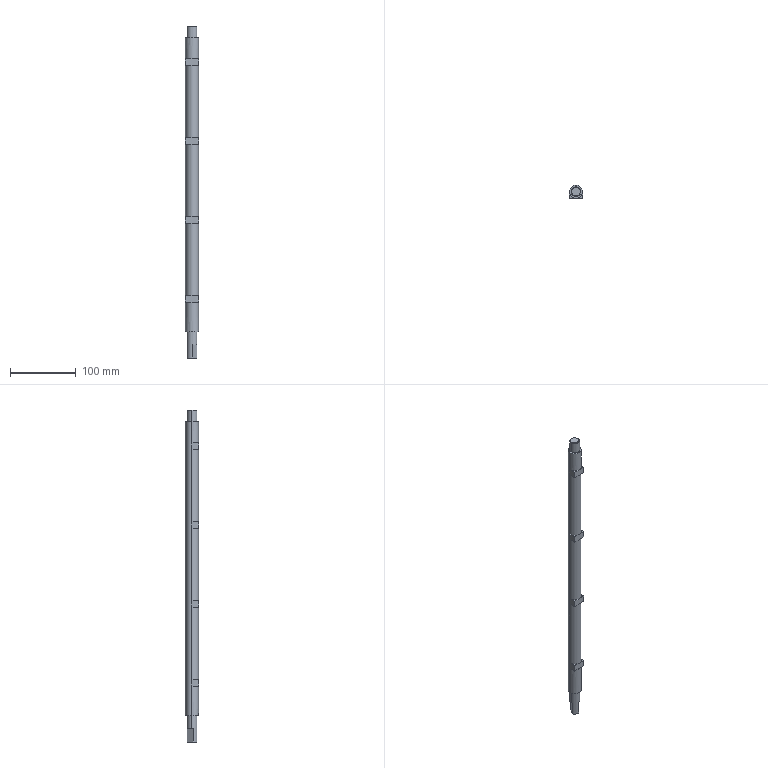Part | SolidWorks | features BaseBody 1 | 1 solid | 48 faces | box 20 x 20 x 505 mm | volume 151599 mm3 | plane 36 | cylinder 10 | cone 2 | commonest cylinder face diameters 20 x6 15 x4
STEP:
#1=CARTESIAN_POINT('',(-1.019,7.43,-20.));
#2=VERTEX_POINT('',#1);
#3=CARTESIAN_POINT('',(-7.5,0.,-20.));
#4=VERTEX_POINT('',#3);
#5=CARTESIAN_POINT('',(0.,0.,-20.));
#6=DIRECTION('',(0.,0.,1.));
#7=DIRECTION('',(1.,0.,0.));
#8=AXIS2_PLACEMENT_3D('',#5,#6,#7);
#9=CIRCLE('',#8,7.5);
#10=EDGE_CURVE('',#2,#4,#9,.T.);
#11=ORIENTED_EDGE('',*,*,#10,.T.);
#12=CARTESIAN_POINT('',(-7.5,0.,0.));
#13=VERTEX_POINT('',#12);
#14=CARTESIAN_POINT('',(-7.5,0.,0.));
#15=DIRECTION('',(0.,0.,1.));
#16=VECTOR('',#15,1000.);
#17=LINE('',#14,#16);
#18=EDGE_CURVE('',#4,#13,#17,.T.);
#19=ORIENTED_EDGE('',*,*,#18,.T.);
#20=CARTESIAN_POINT('',(7.5,0.,0.));
#21=VERTEX_POINT('',#20);
#22=CARTESIAN_POINT('',(0.,0.,0.));
#23=DIRECTION('',(0.,0.,1.));
#24=DIRECTION('',(1.,0.,0.));
#25=AXIS2_PLACEMENT_3D('',#22,#23,#24);
#26=CIRCLE('',#25,7.5);
#27=EDGE_CURVE('',#21,#13,#26,.T.);
#28=ORIENTED_EDGE('',*,*,#27,.F.);
#29=CARTESIAN_POINT('',(7.5,0.,-20.));
#30=VERTEX_POINT('',#29);
#31=CARTESIAN_POINT('',(7.5,0.,0.));
#32=DIRECTION('',(0.,0.,1.));
#33=VECTOR('',#32,1000.);
#34=LINE('',#31,#33);
#35=EDGE_CURVE('',#30,#21,#34,.T.);
#36=ORIENTED_EDGE('',*,*,#35,.F.);
#37=CARTESIAN_POINT('',(7.271,1.838,-20.));
#38=VERTEX_POINT('',#37);
#39=CARTESIAN_POINT('',(0.,0.,-20.));
#40=DIRECTION('',(0.,0.,1.));
#41=DIRECTION('',(1.,0.,0.));
#42=AXIS2_PLACEMENT_3D('',#39,#40,#41);
#43=CIRCLE('',#42,7.5);
#44=EDGE_CURVE('',#30,#38,#43,.T.);
#45=ORIENTED_EDGE('',*,*,#44,.T.);
#46=CARTESIAN_POINT('',(7.271,1.838,-40.));
#47=VERTEX_POINT('',#46);
#48=CARTESIAN_POINT('',(7.271,1.838,0.));
#49=DIRECTION('',(0.,0.,-1.));
#50=VECTOR('',#49,1000.);
#51=LINE('',#48,#50);
#52=EDGE_CURVE('',#38,#47,#51,.T.);
#53=ORIENTED_EDGE('',*,*,#52,.T.);
#54=CARTESIAN_POINT('',(-1.019,7.43,-40.));
#55=VERTEX_POINT('',#54);
#56=CARTESIAN_POINT('',(0.,0.,-40.));
#57=DIRECTION('',(0.,0.,-1.));
#58=DIRECTION('',(1.,0.,0.));
#59=AXIS2_PLACEMENT_3D('',#56,#57,#58);
#60=CIRCLE('',#59,7.5);
#61=EDGE_CURVE('',#55,#47,#60,.T.);
#62=ORIENTED_EDGE('',*,*,#61,.F.);
#63=CARTESIAN_POINT('',(-1.019,7.43,0.));
#64=DIRECTION('',(0.,0.,1.));
#65=VECTOR('',#64,1000.);
#66=LINE('',#63,#65);
#67=EDGE_CURVE('',#55,#2,#66,.T.);
#68=ORIENTED_EDGE('',*,*,#67,.T.);
#69=EDGE_LOOP('',(#11,#19,#28,#36,#45,#53,#62,#68));
#70=FACE_OUTER_BOUND('',#69,.T.);
#71=CARTESIAN_POINT('',(0.,0.,0.));
#72=DIRECTION('',(0.,0.,1.));
#73=DIRECTION('',(1.,0.,0.));
#74=AXIS2_PLACEMENT_3D('',#71,#72,#73);
#75=CYLINDRICAL_SURFACE('',#74,7.5);
#76=ADVANCED_FACE('',(#70),#75,.T.);
#77=CARTESIAN_POINT('',(-6.5,0.,465.));
#78=VERTEX_POINT('',#77);
#79=CARTESIAN_POINT('',(6.5,0.,465.));
#80=VERTEX_POINT('',#79);
#81=CARTESIAN_POINT('',(0.,0.,465.));
#82=DIRECTION('',(0.,0.,-1.));
#83=DIRECTION('',(-1.,0.,0.));
#84=AXIS2_PLACEMENT_3D('',#81,#82,#83);
#85=CIRCLE('',#84,6.5);
#86=EDGE_CURVE('',#78,#80,#85,.T.);
#87=ORIENTED_EDGE('',*,*,#86,.T.);
#88=CARTESIAN_POINT('',(7.5,0.,464.));
#89=VERTEX_POINT('',#88);
#90=CARTESIAN_POINT('',(7.,0.,464.5));
#91=DIRECTION('',(0.7071,0.,-0.7071));
#92=VECTOR('',#91,1000.);
#93=LINE('',#90,#92);
#94=EDGE_CURVE('',#80,#89,#93,.T.);
#95=ORIENTED_EDGE('',*,*,#94,.T.);
#96=CARTESIAN_POINT('',(-7.5,0.,464.));
#97=VERTEX_POINT('',#96);
#98=CARTESIAN_POINT('',(0.,0.,464.));
#99=DIRECTION('',(0.,0.,1.));
#100=DIRECTION('',(-1.,0.,0.));
#101=AXIS2_PLACEMENT_3D('',#98,#99,#100);
#102=CIRCLE('',#101,7.5);
#103=EDGE_CURVE('',#89,#97,#102,.T.);
#104=ORIENTED_EDGE('',*,*,#103,.T.);
#105=CARTESIAN_POINT('',(-7.,0.,464.5));
#106=DIRECTION('',(-0.7071,0.,-0.7071));
#107=VECTOR('',#106,1000.);
#108=LINE('',#105,#107);
#109=EDGE_CURVE('',#78,#97,#108,.T.);
#110=ORIENTED_EDGE('',*,*,#109,.F.);
#111=EDGE_LOOP('',(#87,#95,#104,#110));
#112=FACE_OUTER_BOUND('',#111,.T.);
#113=CARTESIAN_POINT('',(0.,0.,464.5));
#114=DIRECTION('',(0.,0.,-1.));
#115=DIRECTION('',(-1.,0.,0.));
#116=AXIS2_PLACEMENT_3D('',#113,#114,#115);
#117=CONICAL_SURFACE('',#116,7.,0.7854);
#118=ADVANCED_FACE('',(#112),#117,.T.);
#119=ORIENTED_EDGE('',*,*,#103,.F.);
#120=CARTESIAN_POINT('',(7.5,0.,447.));
#121=VERTEX_POINT('',#120);
#122=CARTESIAN_POINT('',(7.5,0.,447.));
#123=DIRECTION('',(0.,0.,-1.));
#124=VECTOR('',#123,1000.);
#125=LINE('',#122,#124);
#126=EDGE_CURVE('',#89,#121,#125,.T.);
#127=ORIENTED_EDGE('',*,*,#126,.T.);
#128=CARTESIAN_POINT('',(-7.5,0.,447.));
#129=VERTEX_POINT('',#128);
#130=CARTESIAN_POINT('',(0.,0.,447.));
#131=DIRECTION('',(0.,0.,-1.));
#132=DIRECTION('',(-1.,0.,0.));
#133=AXIS2_PLACEMENT_3D('',#130,#131,#132);
#134=CIRCLE('',#133,7.5);
#135=EDGE_CURVE('',#129,#121,#134,.T.);
#136=ORIENTED_EDGE('',*,*,#135,.F.);
#137=CARTESIAN_POINT('',(-7.5,0.,447.));
#138=DIRECTION('',(0.,0.,-1.));
#139=VECTOR('',#138,1000.);
#140=LINE('',#137,#139);
#141=EDGE_CURVE('',#97,#129,#140,.T.);
#142=ORIENTED_EDGE('',*,*,#141,.F.);
#143=EDGE_LOOP('',(#119,#127,#136,#142));
#144=FACE_OUTER_BOUND('',#143,.T.);
#145=CARTESIAN_POINT('',(0.,0.,447.));
#146=DIRECTION('',(0.,0.,-1.));
#147=DIRECTION('',(-1.,0.,0.));
#148=AXIS2_PLACEMENT_3D('',#145,#146,#147);
#149=CYLINDRICAL_SURFACE('',#148,7.5);
#150=ADVANCED_FACE('',(#144),#149,.T.);
#151=CARTESIAN_POINT('',(10.,0.,447.));
#152=VERTEX_POINT('',#151);
#153=CARTESIAN_POINT('',(-10.,0.,447.));
#154=VERTEX_POINT('',#153);
#155=CARTESIAN_POINT('',(0.,0.,447.));
#156=DIRECTION('',(0.,0.,1.));
#157=DIRECTION('',(-1.,0.,0.));
#158=AXIS2_PLACEMENT_3D('',#155,#156,#157);
#159=CIRCLE('',#158,10.);
#160=EDGE_CURVE('',#152,#154,#159,.T.);
#161=ORIENTED_EDGE('',*,*,#160,.F.);
#162=CARTESIAN_POINT('',(10.,0.,415.));
#163=VERTEX_POINT('',#162);
#164=CARTESIAN_POINT('',(10.,0.,0.));
#165=DIRECTION('',(0.,0.,-1.));
#166=VECTOR('',#165,1000.);
#167=LINE('',#164,#166);
#168=EDGE_CURVE('',#152,#163,#167,.T.);
#169=ORIENTED_EDGE('',*,*,#168,.T.);
#170=CARTESIAN_POINT('',(10.,0.,405.));
#171=VERTEX_POINT('',#170);
#172=CARTESIAN_POINT('',(10.,0.,0.));
#173=DIRECTION('',(0.,0.,1.));
#174=VECTOR('',#173,1000.);
#175=LINE('',#172,#174);
#176=EDGE_CURVE('',#171,#163,#175,.T.);
#177=ORIENTED_EDGE('',*,*,#176,.F.);
#178=CARTESIAN_POINT('',(10.,0.,295.));
#179=VERTEX_POINT('',#178);
#180=CARTESIAN_POINT('',(10.,0.,0.));
#181=DIRECTION('',(0.,0.,-1.));
#182=VECTOR('',#181,1000.);
#183=LINE('',#180,#182);
#184=EDGE_CURVE('',#171,#179,#183,.T.);
#185=ORIENTED_EDGE('',*,*,#184,.T.);
#186=CARTESIAN_POINT('',(10.,0.,285.));
#187=VERTEX_POINT('',#186);
#188=CARTESIAN_POINT('',(10.,0.,0.));
#189=DIRECTION('',(0.,0.,1.));
#190=VECTOR('',#189,1000.);
#191=LINE('',#188,#190);
#192=EDGE_CURVE('',#187,#179,#191,.T.);
#193=ORIENTED_EDGE('',*,*,#192,.F.);
#194=CARTESIAN_POINT('',(10.,0.,175.));
#195=VERTEX_POINT('',#194);
#196=CARTESIAN_POINT('',(10.,0.,0.));
#197=DIRECTION('',(0.,0.,-1.));
#198=VECTOR('',#197,1000.);
#199=LINE('',#196,#198);
#200=EDGE_CURVE('',#187,#195,#199,.T.);
#201=ORIENTED_EDGE('',*,*,#200,.T.);
#202=CARTESIAN_POINT('',(10.,0.,165.));
#203=VERTEX_POINT('',#202);
#204=CARTESIAN_POINT('',(10.,0.,0.));
#205=DIRECTION('',(0.,0.,1.));
#206=VECTOR('',#205,1000.);
#207=LINE('',#204,#206);
#208=EDGE_CURVE('',#203,#195,#207,.T.);
#209=ORIENTED_EDGE('',*,*,#208,.F.);
#210=CARTESIAN_POINT('',(10.,0.,55.));
#211=VERTEX_POINT('',#210);
#212=CARTESIAN_POINT('',(10.,0.,0.));
#213=DIRECTION('',(0.,0.,-1.));
#214=VECTOR('',#213,1000.);
#215=LINE('',#212,#214);
#216=EDGE_CURVE('',#203,#211,#215,.T.);
#217=ORIENTED_EDGE('',*,*,#216,.T.);
#218=CARTESIAN_POINT('',(10.,0.,45.));
#219=VERTEX_POINT('',#218);
#220=CARTESIAN_POINT('',(10.,0.,0.));
#221=DIRECTION('',(0.,0.,1.));
#222=VECTOR('',#221,1000.);
#223=LINE('',#220,#222);
#224=EDGE_CURVE('',#219,#211,#223,.T.);
#225=ORIENTED_EDGE('',*,*,#224,.F.);
#226=CARTESIAN_POINT('',(10.,0.,0.));
#227=VERTEX_POINT('',#226);
#228=CARTESIAN_POINT('',(10.,0.,0.));
#229=DIRECTION('',(0.,0.,-1.));
#230=VECTOR('',#229,1000.);
#231=LINE('',#228,#230);
#232=EDGE_CURVE('',#219,#227,#231,.T.);
#233=ORIENTED_EDGE('',*,*,#232,.T.);
#234=CARTESIAN_POINT('',(-10.,0.,0.));
#235=VERTEX_POINT('',#234);
#236=CARTESIAN_POINT('',(0.,0.,0.));
#237=DIRECTION('',(0.,0.,-1.));
#238=DIRECTION('',(-1.,0.,0.));
#239=AXIS2_PLACEMENT_3D('',#236,#237,#238);
#240=CIRCLE('',#239,10.);
#241=EDGE_CURVE('',#235,#227,#240,.T.);
#242=ORIENTED_EDGE('',*,*,#241,.F.);
#243=CARTESIAN_POINT('',(-10.,0.,45.));
#244=VERTEX_POINT('',#243);
#245=CARTESIAN_POINT('',(-10.,0.,0.));
#246=DIRECTION('',(0.,0.,-1.));
#247=VECTOR('',#246,1000.);
#248=LINE('',#245,#247);
#249=EDGE_CURVE('',#244,#235,#248,.T.);
#250=ORIENTED_EDGE('',*,*,#249,.F.);
#251=CARTESIAN_POINT('',(-10.,0.,55.));
#252=VERTEX_POINT('',#251);
#253=CARTESIAN_POINT('',(-10.,0.,0.));
#254=DIRECTION('',(0.,0.,1.));
#255=VECTOR('',#254,1000.);
#256=LINE('',#253,#255);
#257=EDGE_CURVE('',#244,#252,#256,.T.);
#258=ORIENTED_EDGE('',*,*,#257,.T.);
#259=CARTESIAN_POINT('',(-10.,0.,165.));
#260=VERTEX_POINT('',#259);
#261=CARTESIAN_POINT('',(-10.,0.,0.));
#262=DIRECTION('',(0.,0.,-1.));
#263=VECTOR('',#262,1000.);
#264=LINE('',#261,#263);
#265=EDGE_CURVE('',#260,#252,#264,.T.);
#266=ORIENTED_EDGE('',*,*,#265,.F.);
#267=CARTESIAN_POINT('',(-10.,0.,175.));
#268=VERTEX_POINT('',#267);
#269=CARTESIAN_POINT('',(-10.,0.,0.));
#270=DIRECTION('',(0.,0.,1.));
#271=VECTOR('',#270,1000.);
#272=LINE('',#269,#271);
#273=EDGE_CURVE('',#260,#268,#272,.T.);
#274=ORIENTED_EDGE('',*,*,#273,.T.);
#275=CARTESIAN_POINT('',(-10.,0.,285.));
#276=VERTEX_POINT('',#275);
#277=CARTESIAN_POINT('',(-10.,0.,0.));
#278=DIRECTION('',(0.,0.,-1.));
#279=VECTOR('',#278,1000.);
#280=LINE('',#277,#279);
#281=EDGE_CURVE('',#276,#268,#280,.T.);
#282=ORIENTED_EDGE('',*,*,#281,.F.);
#283=CARTESIAN_POINT('',(-10.,0.,295.));
#284=VERTEX_POINT('',#283);
#285=CARTESIAN_POINT('',(-10.,0.,0.));
#286=DIRECTION('',(0.,0.,1.));
#287=VECTOR('',#286,1000.);
#288=LINE('',#285,#287);
#289=EDGE_CURVE('',#276,#284,#288,.T.);
#290=ORIENTED_EDGE('',*,*,#289,.T.);
#291=CARTESIAN_POINT('',(-10.,0.,405.));
#292=VERTEX_POINT('',#291);
#293=CARTESIAN_POINT('',(-10.,0.,0.));
#294=DIRECTION('',(0.,0.,-1.));
#295=VECTOR('',#294,1000.);
#296=LINE('',#293,#295);
#297=EDGE_CURVE('',#292,#284,#296,.T.);
#298=ORIENTED_EDGE('',*,*,#297,.F.);
#299=CARTESIAN_POINT('',(-10.,0.,415.));
#300=VERTEX_POINT('',#299);
#301=CARTESIAN_POINT('',(-10.,0.,0.));
#302=DIRECTION('',(0.,0.,1.));
#303=VECTOR('',#302,1000.);
#304=LINE('',#301,#303);
#305=EDGE_CURVE('',#292,#300,#304,.T.);
#306=ORIENTED_EDGE('',*,*,#305,.T.);
#307=CARTESIAN_POINT('',(-10.,0.,0.));
#308=DIRECTION('',(0.,0.,-1.));
#309=VECTOR('',#308,1000.);
#310=LINE('',#307,#309);
#311=EDGE_CURVE('',#154,#300,#310,.T.);
#312=ORIENTED_EDGE('',*,*,#311,.F.);
#313=EDGE_LOOP('',(#161,#169,#177,#185,#193,#201,#209,#217,#225,#233,#242,#250,#258,#266,#274,#282,#290,#298,#306,#312));
#314=FACE_OUTER_BOUND('',#313,.T.);
#315=CARTESIAN_POINT('',(0.,0.,0.));
#316=DIRECTION('',(0.,0.,-1.));
#317=DIRECTION('',(-1.,0.,0.));
#318=AXIS2_PLACEMENT_3D('',#315,#316,#317);
#319=CYLINDRICAL_SURFACE('',#318,10.);
#320=ADVANCED_FACE('',(#314),#319,.T.);
#321=ORIENTED_EDGE('',*,*,#168,.F.);
#322=CARTESIAN_POINT('',(0.,0.,447.));
#323=DIRECTION('',(0.,0.,1.));
#324=DIRECTION('',(-1.,0.,0.));
#325=AXIS2_PLACEMENT_3D('',#322,#323,#324);
#326=CIRCLE('',#325,10.);
#327=EDGE_CURVE('',#154,#152,#326,.T.);
#328=ORIENTED_EDGE('',*,*,#327,.F.);
#329=ORIENTED_EDGE('',*,*,#311,.T.);
#330=CARTESIAN_POINT('',(0.,-10.,415.));
#331=VERTEX_POINT('',#330);
#332=CARTESIAN_POINT('',(0.,0.,415.));
#333=DIRECTION('',(0.,0.,1.));
#334=DIRECTION('',(-1.,0.,0.));
#335=AXIS2_PLACEMENT_3D('',#332,#333,#334);
#336=CIRCLE('',#335,10.);
#337=EDGE_CURVE('',#300,#331,#336,.T.);
#338=ORIENTED_EDGE('',*,*,#337,.T.);
#339=CARTESIAN_POINT('',(0.,0.,415.));
#340=DIRECTION('',(0.,0.,1.));
#341=DIRECTION('',(-1.,0.,0.));
#342=AXIS2_PLACEMENT_3D('',#339,#340,#341);
#343=CIRCLE('',#342,10.);
#344=EDGE_CURVE('',#331,#163,#343,.T.);
#345=ORIENTED_EDGE('',*,*,#344,.T.);
#346=EDGE_LOOP('',(#321,#328,#329,#338,#345));
#347=FACE_OUTER_BOUND('',#346,.T.);
#348=CARTESIAN_POINT('',(0.,0.,0.));
#349=DIRECTION('',(0.,0.,-1.));
#350=DIRECTION('',(-1.,0.,0.));
#351=AXIS2_PLACEMENT_3D('',#348,#349,#350);
#352=CYLINDRICAL_SURFACE('',#351,10.);
#353=ADVANCED_FACE('',(#347),#352,.T.);
#354=ORIENTED_EDGE('',*,*,#184,.F.);
#355=CARTESIAN_POINT('',(0.,-10.,405.));
#356=VERTEX_POINT('',#355);
#357=CARTESIAN_POINT('',(0.,0.,405.));
#358=DIRECTION('',(0.,0.,-1.));
#359=DIRECTION('',(-1.,0.,0.));
#360=AXIS2_PLACEMENT_3D('',#357,#358,#359);
#361=CIRCLE('',#360,10.);
#362=EDGE_CURVE('',#171,#356,#361,.T.);
#363=ORIENTED_EDGE('',*,*,#362,.T.);
#364=CARTESIAN_POINT('',(0.,0.,405.));
#365=DIRECTION('',(0.,0.,-1.));
#366=DIRECTION('',(-1.,0.,0.));
#367=AXIS2_PLACEMENT_3D('',#364,#365,#366);
#368=CIRCLE('',#367,10.);
#369=EDGE_CURVE('',#356,#292,#368,.T.);
#370=ORIENTED_EDGE('',*,*,#369,.T.);
#371=ORIENTED_EDGE('',*,*,#297,.T.);
#372=CARTESIAN_POINT('',(0.,-10.,295.));
#373=VERTEX_POINT('',#372);
#374=CARTESIAN_POINT('',(0.,0.,295.));
#375=DIRECTION('',(0.,0.,1.));
#376=DIRECTION('',(-1.,0.,0.));
#377=AXIS2_PLACEMENT_3D('',#374,#375,#376);
#378=CIRCLE('',#377,10.);
#379=EDGE_CURVE('',#284,#373,#378,.T.);
#380=ORIENTED_EDGE('',*,*,#379,.T.);
#381=CARTESIAN_POINT('',(0.,0.,295.));
#382=DIRECTION('',(0.,0.,1.));
#383=DIRECTION('',(-1.,0.,0.));
#384=AXIS2_PLACEMENT_3D('',#381,#382,#383);
#385=CIRCLE('',#384,10.);
#386=EDGE_CURVE('',#373,#179,#385,.T.);
#387=ORIENTED_EDGE('',*,*,#386,.T.);
#388=EDGE_LOOP('',(#354,#363,#370,#371,#380,#387));
#389=FACE_OUTER_BOUND('',#388,.T.);
#390=CARTESIAN_POINT('',(0.,0.,0.));
#391=DIRECTION('',(0.,0.,-1.));
#392=DIRECTION('',(-1.,0.,0.));
#393=AXIS2_PLACEMENT_3D('',#390,#391,#392);
#394=CYLINDRICAL_SURFACE('',#393,10.);
#395=ADVANCED_FACE('',(#389),#394,.T.);
#396=ORIENTED_EDGE('',*,*,#200,.F.);
#397=CARTESIAN_POINT('',(0.,-10.,285.));
#398=VERTEX_POINT('',#397);
#399=CARTESIAN_POINT('',(0.,0.,285.));
#400=DIRECTION('',(0.,0.,-1.));
#401=DIRECTION('',(-1.,0.,0.));
#402=AXIS2_PLACEMENT_3D('',#399,#400,#401);
#403=CIRCLE('',#402,10.);
#404=EDGE_CURVE('',#187,#398,#403,.T.);
#405=ORIENTED_EDGE('',*,*,#404,.T.);
#406=CARTESIAN_POINT('',(0.,0.,285.));
#407=DIRECTION('',(0.,0.,-1.));
#408=DIRECTION('',(-1.,0.,0.));
#409=AXIS2_PLACEMENT_3D('',#406,#407,#408);
#410=CIRCLE('',#409,10.);
#411=EDGE_CURVE('',#398,#276,#410,.T.);
#412=ORIENTED_EDGE('',*,*,#411,.T.);
#413=ORIENTED_EDGE('',*,*,#281,.T.);
#414=CARTESIAN_POINT('',(0.,-10.,175.));
#415=VERTEX_POINT('',#414);
#416=CARTESIAN_POINT('',(0.,0.,175.));
#417=DIRECTION('',(0.,0.,1.));
#418=DIRECTION('',(-1.,0.,0.));
#419=AXIS2_PLACEMENT_3D('',#416,#417,#418);
#420=CIRCLE('',#419,10.);
#421=EDGE_CURVE('',#268,#415,#420,.T.);
#422=ORIENTED_EDGE('',*,*,#421,.T.);
#423=CARTESIAN_POINT('',(0.,0.,175.));
#424=DIRECTION('',(0.,0.,1.));
#425=DIRECTION('',(-1.,0.,0.));
#426=AXIS2_PLACEMENT_3D('',#423,#424,#425);
#427=CIRCLE('',#426,10.);
#428=EDGE_CURVE('',#415,#195,#427,.T.);
#429=ORIENTED_EDGE('',*,*,#428,.T.);
#430=EDGE_LOOP('',(#396,#405,#412,#413,#422,#429));
#431=FACE_OUTER_BOUND('',#430,.T.);
#432=CARTESIAN_POINT('',(0.,0.,0.));
#433=DIRECTION('',(0.,0.,-1.));
#434=DIRECTION('',(-1.,0.,0.));
#435=AXIS2_PLACEMENT_3D('',#432,#433,#434);
#436=CYLINDRICAL_SURFACE('',#435,10.);
#437=ADVANCED_FACE('',(#431),#436,.T.);
#438=ORIENTED_EDGE('',*,*,#216,.F.);
#439=CARTESIAN_POINT('',(0.,-10.,165.));
#440=VERTEX_POINT('',#439);
#441=CARTESIAN_POINT('',(0.,0.,165.));
#442=DIRECTION('',(0.,0.,-1.));
#443=DIRECTION('',(-1.,0.,0.));
#444=AXIS2_PLACEMENT_3D('',#441,#442,#443);
#445=CIRCLE('',#444,10.);
#446=EDGE_CURVE('',#203,#440,#445,.T.);
#447=ORIENTED_EDGE('',*,*,#446,.T.);
#448=CARTESIAN_POINT('',(0.,0.,165.));
#449=DIRECTION('',(0.,0.,-1.));
#450=DIRECTION('',(-1.,0.,0.));
#451=AXIS2_PLACEMENT_3D('',#448,#449,#450);
#452=CIRCLE('',#451,10.);
#453=EDGE_CURVE('',#440,#260,#452,.T.);
#454=ORIENTED_EDGE('',*,*,#453,.T.);
#455=ORIENTED_EDGE('',*,*,#265,.T.);
#456=CARTESIAN_POINT('',(0.,-10.,55.));
#457=VERTEX_POINT('',#456);
#458=CARTESIAN_POINT('',(0.,0.,55.));
#459=DIRECTION('',(0.,0.,1.));
#460=DIRECTION('',(-1.,0.,0.));
#461=AXIS2_PLACEMENT_3D('',#458,#459,#460);
#462=CIRCLE('',#461,10.);
#463=EDGE_CURVE('',#252,#457,#462,.T.);
#464=ORIENTED_EDGE('',*,*,#463,.T.);
#465=CARTESIAN_POINT('',(0.,0.,55.));
#466=DIRECTION('',(0.,0.,1.));
#467=DIRECTION('',(-1.,0.,0.));
#468=AXIS2_PLACEMENT_3D('',#465,#466,#467);
#469=CIRCLE('',#468,10.);
#470=EDGE_CURVE('',#457,#211,#469,.T.);
#471=ORIENTED_EDGE('',*,*,#470,.T.);
#472=EDGE_LOOP('',(#438,#447,#454,#455,#464,#471));
#473=FACE_OUTER_BOUND('',#472,.T.);
#474=CARTESIAN_POINT('',(0.,0.,0.));
#475=DIRECTION('',(0.,0.,-1.));
#476=DIRECTION('',(-1.,0.,0.));
#477=AXIS2_PLACEMENT_3D('',#474,#475,#476);
#478=CYLINDRICAL_SURFACE('',#477,10.);
#479=ADVANCED_FACE('',(#473),#478,.T.);
#480=CARTESIAN_POINT('',(-7.271,-1.838,-40.));
#481=VERTEX_POINT('',#480);
#482=CARTESIAN_POINT('',(-5.708,0.4787,-40.));
#483=DIRECTION('',(0.5592,0.829,0.));
#484=VECTOR('',#483,1000.);
#485=LINE('',#482,#484);
#486=EDGE_CURVE('',#481,#55,#485,.T.);
#487=ORIENTED_EDGE('',*,*,#486,.F.);
#488=CARTESIAN_POINT('',(-7.271,-1.838,-20.));
#489=VERTEX_POINT('',#488);
#490=CARTESIAN_POINT('',(-7.271,-1.838,0.));
#491=DIRECTION('',(0.,0.,-1.));
#492=VECTOR('',#491,1000.);
#493=LINE('',#490,#492);
#494=EDGE_CURVE('',#489,#481,#493,.T.);
#495=ORIENTED_EDGE('',*,*,#494,.F.);
#496=CARTESIAN_POINT('',(-1.019,7.43,-20.));
#497=DIRECTION('',(0.5592,0.829,0.));
#498=VECTOR('',#497,1000.);
#499=LINE('',#496,#498);
#500=EDGE_CURVE('',#489,#2,#499,.T.);
#501=ORIENTED_EDGE('',*,*,#500,.T.);
#502=ORIENTED_EDGE('',*,*,#67,.F.);
#503=EDGE_LOOP('',(#487,#495,#501,#502));
#504=FACE_OUTER_BOUND('',#503,.T.);
#505=CARTESIAN_POINT('',(-7.271,-1.838,-40.));
#506=DIRECTION('',(0.829,-0.5592,0.));
#507=DIRECTION('',(0.,0.,-1.));
#508=AXIS2_PLACEMENT_3D('',#505,#506,#507);
#509=PLANE('',#508);
#510=ADVANCED_FACE('',(#504),#509,.F.);
#511=ORIENTED_EDGE('',*,*,#10,.F.);
#512=ORIENTED_EDGE('',*,*,#500,.F.);
#513=CARTESIAN_POINT('',(0.,0.,-20.));
#514=DIRECTION('',(0.,0.,1.));
#515=DIRECTION('',(1.,0.,0.));
#516=AXIS2_PLACEMENT_3D('',#513,#514,#515);
#517=CIRCLE('',#516,7.5);
#518=EDGE_CURVE('',#4,#489,#517,.T.);
#519=ORIENTED_EDGE('',*,*,#518,.F.);
#520=EDGE_LOOP('',(#511,#512,#519));
#521=FACE_OUTER_BOUND('',#520,.T.);
#522=CARTESIAN_POINT('',(-4.771,3.218,-20.));
#523=DIRECTION('',(0.,0.,1.));
#524=DIRECTION('',(1.,0.,0.));
#525=AXIS2_PLACEMENT_3D('',#522,#523,#524);
#526=PLANE('',#525);
#527=ADVANCED_FACE('',(#521),#526,.F.);
#528=CARTESIAN_POINT('',(1.019,-7.43,-40.));
#529=VERTEX_POINT('',#528);
#530=CARTESIAN_POINT('',(5.708,-0.4787,-40.));
#531=DIRECTION('',(-0.5592,-0.829,0.));
#532=VECTOR('',#531,1000.);
#533=LINE('',#530,#532);
#534=EDGE_CURVE('',#47,#529,#533,.T.);
#535=ORIENTED_EDGE('',*,*,#534,.F.);
#536=ORIENTED_EDGE('',*,*,#52,.F.);
#537=CARTESIAN_POINT('',(1.019,-7.43,-20.));
#538=VERTEX_POINT('',#537);
#539=CARTESIAN_POINT('',(1.019,-7.43,-20.));
#540=DIRECTION('',(-0.5592,-0.829,0.));
#541=VECTOR('',#540,1000.);
#542=LINE('',#539,#541);
#543=EDGE_CURVE('',#38,#538,#542,.T.);
#544=ORIENTED_EDGE('',*,*,#543,.T.);
#545=CARTESIAN_POINT('',(1.019,-7.43,0.));
#546=DIRECTION('',(0.,0.,1.));
#547=VECTOR('',#546,1000.);
#548=LINE('',#545,#547);
#549=EDGE_CURVE('',#529,#538,#548,.T.);
#550=ORIENTED_EDGE('',*,*,#549,.F.);
#551=EDGE_LOOP('',(#535,#536,#544,#550));
#552=FACE_OUTER_BOUND('',#551,.T.);
#553=CARTESIAN_POINT('',(7.271,1.838,-40.));
#554=DIRECTION('',(-0.829,0.5592,0.));
#555=DIRECTION('',(0.,0.,1.));
#556=AXIS2_PLACEMENT_3D('',#553,#554,#555);
#557=PLANE('',#556);
#558=ADVANCED_FACE('',(#552),#557,.F.);
#559=ORIENTED_EDGE('',*,*,#543,.F.);
#560=ORIENTED_EDGE('',*,*,#44,.F.);
#561=CARTESIAN_POINT('',(0.,0.,-20.));
#562=DIRECTION('',(0.,0.,1.));
#563=DIRECTION('',(1.,0.,0.));
#564=AXIS2_PLACEMENT_3D('',#561,#562,#563);
#565=CIRCLE('',#564,7.5);
#566=EDGE_CURVE('',#538,#30,#565,.T.);
#567=ORIENTED_EDGE('',*,*,#566,.F.);
#568=EDGE_LOOP('',(#559,#560,#567));
#569=FACE_OUTER_BOUND('',#568,.T.);
#570=CARTESIAN_POINT('',(4.771,-3.218,-20.));
#571=DIRECTION('',(0.,0.,1.));
#572=DIRECTION('',(1.,0.,0.));
#573=AXIS2_PLACEMENT_3D('',#570,#571,#572);
#574=PLANE('',#573);
#575=ADVANCED_FACE('',(#569),#574,.F.);
#576=ORIENTED_EDGE('',*,*,#486,.T.);
#577=ORIENTED_EDGE('',*,*,#61,.T.);
#578=ORIENTED_EDGE('',*,*,#534,.T.);
#579=CARTESIAN_POINT('',(0.,0.,-40.));
#580=DIRECTION('',(0.,0.,-1.));
#581=DIRECTION('',(1.,0.,0.));
#582=AXIS2_PLACEMENT_3D('',#579,#580,#581);
#583=CIRCLE('',#582,7.5);
#584=EDGE_CURVE('',#529,#481,#583,.T.);
#585=ORIENTED_EDGE('',*,*,#584,.T.);
#586=EDGE_LOOP('',(#576,#577,#578,#585));
#587=FACE_OUTER_BOUND('',#586,.T.);
#588=CARTESIAN_POINT('',(0.,0.,-40.));
#589=DIRECTION('',(0.,0.,1.));
#590=DIRECTION('',(1.,0.,0.));
#591=AXIS2_PLACEMENT_3D('',#588,#589,#590);
#592=PLANE('',#591);
#593=ADVANCED_FACE('',(#587),#592,.F.);
#594=ORIENTED_EDGE('',*,*,#337,.F.);
#595=CARTESIAN_POINT('',(-10.,-10.,415.));
#596=VERTEX_POINT('',#595);
#597=CARTESIAN_POINT('',(-10.,-10.,415.));
#598=DIRECTION('',(0.,-1.,0.));
#599=VECTOR('',#598,1000.);
#600=LINE('',#597,#599);
#601=EDGE_CURVE('',#300,#596,#600,.T.);
#602=ORIENTED_EDGE('',*,*,#601,.T.);
#603=CARTESIAN_POINT('',(10.,-10.,415.));
#604=DIRECTION('',(1.,0.,0.));
#605=VECTOR('',#604,1000.);
#606=LINE('',#603,#605);
#607=EDGE_CURVE('',#596,#331,#606,.T.);
#608=ORIENTED_EDGE('',*,*,#607,.T.);
#609=EDGE_LOOP('',(#594,#602,#608));
#610=FACE_OUTER_BOUND('',#609,.T.);
#611=CARTESIAN_POINT('',(0.,-2.36,415.));
#612=DIRECTION('',(0.,0.,1.));
#613=DIRECTION('',(1.,0.,0.));
#614=AXIS2_PLACEMENT_3D('',#611,#612,#613);
#615=PLANE('',#614);
#616=ADVANCED_FACE('',(#610),#615,.T.);
#617=ORIENTED_EDGE('',*,*,#344,.F.);
#618=CARTESIAN_POINT('',(10.,-10.,415.));
#619=VERTEX_POINT('',#618);
#620=CARTESIAN_POINT('',(10.,-10.,415.));
#621=DIRECTION('',(1.,0.,0.));
#622=VECTOR('',#621,1000.);
#623=LINE('',#620,#622);
#624=EDGE_CURVE('',#331,#619,#623,.T.);
#625=ORIENTED_EDGE('',*,*,#624,.T.);
#626=CARTESIAN_POINT('',(10.,0.,415.));
#627=DIRECTION('',(0.,1.,0.));
#628=VECTOR('',#627,1000.);
#629=LINE('',#626,#628);
#630=EDGE_CURVE('',#619,#163,#629,.T.);
#631=ORIENTED_EDGE('',*,*,#630,.T.);
#632=EDGE_LOOP('',(#617,#625,#631));
#633=FACE_OUTER_BOUND('',#632,.T.);
#634=CARTESIAN_POINT('',(0.,-2.36,415.));
#635=DIRECTION('',(0.,0.,1.));
#636=DIRECTION('',(1.,0.,0.));
#637=AXIS2_PLACEMENT_3D('',#634,#635,#636);
#638=PLANE('',#637);
#639=ADVANCED_FACE('',(#633),#638,.T.);
#640=ORIENTED_EDGE('',*,*,#369,.F.);
#641=CARTESIAN_POINT('',(-10.,-10.,405.));
#642=VERTEX_POINT('',#641);
#643=CARTESIAN_POINT('',(10.,-10.,405.));
#644=DIRECTION('',(-1.,0.,0.));
#645=VECTOR('',#644,1000.);
#646=LINE('',#643,#645);
#647=EDGE_CURVE('',#356,#642,#646,.T.);
#648=ORIENTED_EDGE('',*,*,#647,.T.);
#649=CARTESIAN_POINT('',(-10.,-10.,405.));
#650=DIRECTION('',(0.,1.,0.));
#651=VECTOR('',#650,1000.);
#652=LINE('',#649,#651);
#653=EDGE_CURVE('',#642,#292,#652,.T.);
#654=ORIENTED_EDGE('',*,*,#653,.T.);
#655=EDGE_LOOP('',(#640,#648,#654));
#656=FACE_OUTER_BOUND('',#655,.T.);
#657=CARTESIAN_POINT('',(0.,-2.36,405.));
#658=DIRECTION('',(0.,0.,1.));
#659=DIRECTION('',(1.,0.,0.));
#660=AXIS2_PLACEMENT_3D('',#657,#658,#659);
#661=PLANE('',#660);
#662=ADVANCED_FACE('',(#656),#661,.F.);
#663=ORIENTED_EDGE('',*,*,#653,.F.);
#664=CARTESIAN_POINT('',(-10.,-10.,405.));
#665=DIRECTION('',(0.,0.,1.));
#666=VECTOR('',#665,1000.);
#667=LINE('',#664,#666);
#668=EDGE_CURVE('',#642,#596,#667,.T.);
#669=ORIENTED_EDGE('',*,*,#668,.T.);
#670=ORIENTED_EDGE('',*,*,#601,.F.);
#671=ORIENTED_EDGE('',*,*,#305,.F.);
#672=EDGE_LOOP('',(#663,#669,#670,#671));
#673=FACE_OUTER_BOUND('',#672,.T.);
#674=CARTESIAN_POINT('',(-10.,0.,405.));
#675=DIRECTION('',(-1.,0.,0.));
#676=DIRECTION('',(0.,0.,1.));
#677=AXIS2_PLACEMENT_3D('',#674,#675,#676);
#678=PLANE('',#677);
#679=ADVANCED_FACE('',(#673),#678,.T.);
#680=CARTESIAN_POINT('',(10.,-10.,405.));
#681=VERTEX_POINT('',#680);
#682=CARTESIAN_POINT('',(10.,0.,405.));
#683=DIRECTION('',(0.,-1.,0.));
#684=VECTOR('',#683,1000.);
#685=LINE('',#682,#684);
#686=EDGE_CURVE('',#171,#681,#685,.T.);
#687=ORIENTED_EDGE('',*,*,#686,.F.);
#688=ORIENTED_EDGE('',*,*,#176,.T.);
#689=ORIENTED_EDGE('',*,*,#630,.F.);
#690=CARTESIAN_POINT('',(10.,-10.,405.));
#691=DIRECTION('',(0.,0.,1.));
#692=VECTOR('',#691,1000.);
#693=LINE('',#690,#692);
#694=EDGE_CURVE('',#681,#619,#693,.T.);
#695=ORIENTED_EDGE('',*,*,#694,.F.);
#696=EDGE_LOOP('',(#687,#688,#689,#695));
#697=FACE_OUTER_BOUND('',#696,.T.);
#698=CARTESIAN_POINT('',(10.,-10.,405.));
#699=DIRECTION('',(1.,0.,0.));
#700=DIRECTION('',(0.,-1.,0.));
#701=AXIS2_PLACEMENT_3D('',#698,#699,#700);
#702=PLANE('',#701);
#703=ADVANCED_FACE('',(#697),#702,.T.);
#704=ORIENTED_EDGE('',*,*,#607,.F.);
#705=ORIENTED_EDGE('',*,*,#668,.F.);
#706=ORIENTED_EDGE('',*,*,#647,.F.);
#707=CARTESIAN_POINT('',(10.,-10.,405.));
#708=DIRECTION('',(-1.,0.,0.));
#709=VECTOR('',#708,1000.);
#710=LINE('',#707,#709);
#711=EDGE_CURVE('',#681,#356,#710,.T.);
#712=ORIENTED_EDGE('',*,*,#711,.F.);
#713=ORIENTED_EDGE('',*,*,#694,.T.);
#714=ORIENTED_EDGE('',*,*,#624,.F.);
#715=EDGE_LOOP('',(#704,#705,#706,#712,#713,#714));
#716=FACE_OUTER_BOUND('',#715,.T.);
#717=CARTESIAN_POINT('',(-10.,-10.,405.));
#718=DIRECTION('',(0.,-1.,0.));
#719=DIRECTION('',(0.,0.,-1.));
#720=AXIS2_PLACEMENT_3D('',#717,#718,#719);
#721=PLANE('',#720);
#722=ADVANCED_FACE('',(#716),#721,.T.);
#723=ORIENTED_EDGE('',*,*,#362,.F.);
#724=ORIENTED_EDGE('',*,*,#686,.T.);
#725=ORIENTED_EDGE('',*,*,#711,.T.);
#726=EDGE_LOOP('',(#723,#724,#725));
#727=FACE_OUTER_BOUND('',#726,.T.);
#728=CARTESIAN_POINT('',(0.,-2.36,405.));
#729=DIRECTION('',(0.,0.,1.));
#730=DIRECTION('',(1.,0.,0.));
#731=AXIS2_PLACEMENT_3D('',#728,#729,#730);
#732=PLANE('',#731);
#733=ADVANCED_FACE('',(#727),#732,.F.);
#734=ORIENTED_EDGE('',*,*,#379,.F.);
#735=CARTESIAN_POINT('',(-10.,-10.,295.));
#736=VERTEX_POINT('',#735);
#737=CARTESIAN_POINT('',(-10.,-10.,295.));
#738=DIRECTION('',(0.,-1.,0.));
#739=VECTOR('',#738,1000.);
#740=LINE('',#737,#739);
#741=EDGE_CURVE('',#284,#736,#740,.T.);
#742=ORIENTED_EDGE('',*,*,#741,.T.);
#743=CARTESIAN_POINT('',(10.,-10.,295.));
#744=DIRECTION('',(1.,0.,0.));
#745=VECTOR('',#744,1000.);
#746=LINE('',#743,#745);
#747=EDGE_CURVE('',#736,#373,#746,.T.);
#748=ORIENTED_EDGE('',*,*,#747,.T.);
#749=EDGE_LOOP('',(#734,#742,#748));
#750=FACE_OUTER_BOUND('',#749,.T.);
#751=CARTESIAN_POINT('',(0.,-2.36,295.));
#752=DIRECTION('',(0.,0.,1.));
#753=DIRECTION('',(1.,0.,0.));
#754=AXIS2_PLACEMENT_3D('',#751,#752,#753);
#755=PLANE('',#754);
#756=ADVANCED_FACE('',(#750),#755,.T.);
#757=ORIENTED_EDGE('',*,*,#386,.F.);
#758=CARTESIAN_POINT('',(10.,-10.,295.));
#759=VERTEX_POINT('',#758);
#760=CARTESIAN_POINT('',(10.,-10.,295.));
#761=DIRECTION('',(1.,0.,0.));
#762=VECTOR('',#761,1000.);
#763=LINE('',#760,#762);
#764=EDGE_CURVE('',#373,#759,#763,.T.);
#765=ORIENTED_EDGE('',*,*,#764,.T.);
#766=CARTESIAN_POINT('',(10.,0.,295.));
#767=DIRECTION('',(0.,1.,0.));
#768=VECTOR('',#767,1000.);
#769=LINE('',#766,#768);
#770=EDGE_CURVE('',#759,#179,#769,.T.);
#771=ORIENTED_EDGE('',*,*,#770,.T.);
#772=EDGE_LOOP('',(#757,#765,#771));
#773=FACE_OUTER_BOUND('',#772,.T.);
#774=CARTESIAN_POINT('',(0.,-2.36,295.));
#775=DIRECTION('',(0.,0.,1.));
#776=DIRECTION('',(1.,0.,0.));
#777=AXIS2_PLACEMENT_3D('',#774,#775,#776);
#778=PLANE('',#777);
#779=ADVANCED_FACE('',(#773),#778,.T.);
#780=ORIENTED_EDGE('',*,*,#411,.F.);
#781=CARTESIAN_POINT('',(-10.,-10.,285.));
#782=VERTEX_POINT('',#781);
#783=CARTESIAN_POINT('',(10.,-10.,285.));
#784=DIRECTION('',(-1.,0.,0.));
#785=VECTOR('',#784,1000.);
#786=LINE('',#783,#785);
#787=EDGE_CURVE('',#398,#782,#786,.T.);
#788=ORIENTED_EDGE('',*,*,#787,.T.);
#789=CARTESIAN_POINT('',(-10.,-10.,285.));
#790=DIRECTION('',(0.,1.,0.));
#791=VECTOR('',#790,1000.);
#792=LINE('',#789,#791);
#793=EDGE_CURVE('',#782,#276,#792,.T.);
#794=ORIENTED_EDGE('',*,*,#793,.T.);
#795=EDGE_LOOP('',(#780,#788,#794));
#796=FACE_OUTER_BOUND('',#795,.T.);
#797=CARTESIAN_POINT('',(0.,-2.36,285.));
#798=DIRECTION('',(0.,0.,1.));
#799=DIRECTION('',(1.,0.,0.));
#800=AXIS2_PLACEMENT_3D('',#797,#798,#799);
#801=PLANE('',#800);
#802=ADVANCED_FACE('',(#796),#801,.F.);
#803=ORIENTED_EDGE('',*,*,#793,.F.);
#804=CARTESIAN_POINT('',(-10.,-10.,285.));
#805=DIRECTION('',(0.,0.,1.));
#806=VECTOR('',#805,1000.);
#807=LINE('',#804,#806);
#808=EDGE_CURVE('',#782,#736,#807,.T.);
#809=ORIENTED_EDGE('',*,*,#808,.T.);
#810=ORIENTED_EDGE('',*,*,#741,.F.);
#811=ORIENTED_EDGE('',*,*,#289,.F.);
#812=EDGE_LOOP('',(#803,#809,#810,#811));
#813=FACE_OUTER_BOUND('',#812,.T.);
#814=CARTESIAN_POINT('',(-10.,0.,285.));
#815=DIRECTION('',(-1.,0.,0.));
#816=DIRECTION('',(0.,0.,1.));
#817=AXIS2_PLACEMENT_3D('',#814,#815,#816);
#818=PLANE('',#817);
#819=ADVANCED_FACE('',(#813),#818,.T.);
#820=CARTESIAN_POINT('',(10.,-10.,285.));
#821=VERTEX_POINT('',#820);
#822=CARTESIAN_POINT('',(10.,0.,285.));
#823=DIRECTION('',(0.,-1.,0.));
#824=VECTOR('',#823,1000.);
#825=LINE('',#822,#824);
#826=EDGE_CURVE('',#187,#821,#825,.T.);
#827=ORIENTED_EDGE('',*,*,#826,.F.);
#828=ORIENTED_EDGE('',*,*,#192,.T.);
#829=ORIENTED_EDGE('',*,*,#770,.F.);
#830=CARTESIAN_POINT('',(10.,-10.,285.));
#831=DIRECTION('',(0.,0.,1.));
#832=VECTOR('',#831,1000.);
#833=LINE('',#830,#832);
#834=EDGE_CURVE('',#821,#759,#833,.T.);
#835=ORIENTED_EDGE('',*,*,#834,.F.);
#836=EDGE_LOOP('',(#827,#828,#829,#835));
#837=FACE_OUTER_BOUND('',#836,.T.);
#838=CARTESIAN_POINT('',(10.,-10.,285.));
#839=DIRECTION('',(1.,0.,0.));
#840=DIRECTION('',(0.,-1.,0.));
#841=AXIS2_PLACEMENT_3D('',#838,#839,#840);
#842=PLANE('',#841);
#843=ADVANCED_FACE('',(#837),#842,.T.);
#844=ORIENTED_EDGE('',*,*,#747,.F.);
#845=ORIENTED_EDGE('',*,*,#808,.F.);
#846=ORIENTED_EDGE('',*,*,#787,.F.);
#847=CARTESIAN_POINT('',(10.,-10.,285.));
#848=DIRECTION('',(-1.,0.,0.));
#849=VECTOR('',#848,1000.);
#850=LINE('',#847,#849);
#851=EDGE_CURVE('',#821,#398,#850,.T.);
#852=ORIENTED_EDGE('',*,*,#851,.F.);
#853=ORIENTED_EDGE('',*,*,#834,.T.);
#854=ORIENTED_EDGE('',*,*,#764,.F.);
#855=EDGE_LOOP('',(#844,#845,#846,#852,#853,#854));
#856=FACE_OUTER_BOUND('',#855,.T.);
#857=CARTESIAN_POINT('',(-10.,-10.,285.));
#858=DIRECTION('',(0.,-1.,0.));
#859=DIRECTION('',(0.,0.,-1.));
#860=AXIS2_PLACEMENT_3D('',#857,#858,#859);
#861=PLANE('',#860);
#862=ADVANCED_FACE('',(#856),#861,.T.);
#863=ORIENTED_EDGE('',*,*,#404,.F.);
#864=ORIENTED_EDGE('',*,*,#826,.T.);
#865=ORIENTED_EDGE('',*,*,#851,.T.);
#866=EDGE_LOOP('',(#863,#864,#865));
#867=FACE_OUTER_BOUND('',#866,.T.);
#868=CARTESIAN_POINT('',(0.,-2.36,285.));
#869=DIRECTION('',(0.,0.,1.));
#870=DIRECTION('',(1.,0.,0.));
#871=AXIS2_PLACEMENT_3D('',#868,#869,#870);
#872=PLANE('',#871);
#873=ADVANCED_FACE('',(#867),#872,.F.);
#874=ORIENTED_EDGE('',*,*,#421,.F.);
#875=CARTESIAN_POINT('',(-10.,-10.,175.));
#876=VERTEX_POINT('',#875);
#877=CARTESIAN_POINT('',(-10.,-10.,175.));
#878=DIRECTION('',(0.,-1.,0.));
#879=VECTOR('',#878,1000.);
#880=LINE('',#877,#879);
#881=EDGE_CURVE('',#268,#876,#880,.T.);
#882=ORIENTED_EDGE('',*,*,#881,.T.);
#883=CARTESIAN_POINT('',(10.,-10.,175.));
#884=DIRECTION('',(1.,0.,0.));
#885=VECTOR('',#884,1000.);
#886=LINE('',#883,#885);
#887=EDGE_CURVE('',#876,#415,#886,.T.);
#888=ORIENTED_EDGE('',*,*,#887,.T.);
#889=EDGE_LOOP('',(#874,#882,#888));
#890=FACE_OUTER_BOUND('',#889,.T.);
#891=CARTESIAN_POINT('',(0.,-2.36,175.));
#892=DIRECTION('',(0.,0.,1.));
#893=DIRECTION('',(1.,0.,0.));
#894=AXIS2_PLACEMENT_3D('',#891,#892,#893);
#895=PLANE('',#894);
#896=ADVANCED_FACE('',(#890),#895,.T.);
#897=ORIENTED_EDGE('',*,*,#428,.F.);
#898=CARTESIAN_POINT('',(10.,-10.,175.));
#899=VERTEX_POINT('',#898);
#900=CARTESIAN_POINT('',(10.,-10.,175.));
#901=DIRECTION('',(1.,0.,0.));
#902=VECTOR('',#901,1000.);
#903=LINE('',#900,#902);
#904=EDGE_CURVE('',#415,#899,#903,.T.);
#905=ORIENTED_EDGE('',*,*,#904,.T.);
#906=CARTESIAN_POINT('',(10.,0.,175.));
#907=DIRECTION('',(0.,1.,0.));
#908=VECTOR('',#907,1000.);
#909=LINE('',#906,#908);
#910=EDGE_CURVE('',#899,#195,#909,.T.);
#911=ORIENTED_EDGE('',*,*,#910,.T.);
#912=EDGE_LOOP('',(#897,#905,#911));
#913=FACE_OUTER_BOUND('',#912,.T.);
#914=CARTESIAN_POINT('',(0.,-2.36,175.));
#915=DIRECTION('',(0.,0.,1.));
#916=DIRECTION('',(1.,0.,0.));
#917=AXIS2_PLACEMENT_3D('',#914,#915,#916);
#918=PLANE('',#917);
#919=ADVANCED_FACE('',(#913),#918,.T.);
#920=ORIENTED_EDGE('',*,*,#453,.F.);
#921=CARTESIAN_POINT('',(-10.,-10.,165.));
#922=VERTEX_POINT('',#921);
#923=CARTESIAN_POINT('',(10.,-10.,165.));
#924=DIRECTION('',(-1.,0.,0.));
#925=VECTOR('',#924,1000.);
#926=LINE('',#923,#925);
#927=EDGE_CURVE('',#440,#922,#926,.T.);
#928=ORIENTED_EDGE('',*,*,#927,.T.);
#929=CARTESIAN_POINT('',(-10.,-10.,165.));
#930=DIRECTION('',(0.,1.,0.));
#931=VECTOR('',#930,1000.);
#932=LINE('',#929,#931);
#933=EDGE_CURVE('',#922,#260,#932,.T.);
#934=ORIENTED_EDGE('',*,*,#933,.T.);
#935=EDGE_LOOP('',(#920,#928,#934));
#936=FACE_OUTER_BOUND('',#935,.T.);
#937=CARTESIAN_POINT('',(0.,-2.36,165.));
#938=DIRECTION('',(0.,0.,1.));
#939=DIRECTION('',(1.,0.,0.));
#940=AXIS2_PLACEMENT_3D('',#937,#938,#939);
#941=PLANE('',#940);
#942=ADVANCED_FACE('',(#936),#941,.F.);
#943=ORIENTED_EDGE('',*,*,#933,.F.);
#944=CARTESIAN_POINT('',(-10.,-10.,165.));
#945=DIRECTION('',(0.,0.,1.));
#946=VECTOR('',#945,1000.);
#947=LINE('',#944,#946);
#948=EDGE_CURVE('',#922,#876,#947,.T.);
#949=ORIENTED_EDGE('',*,*,#948,.T.);
#950=ORIENTED_EDGE('',*,*,#881,.F.);
#951=ORIENTED_EDGE('',*,*,#273,.F.);
#952=EDGE_LOOP('',(#943,#949,#950,#951));
#953=FACE_OUTER_BOUND('',#952,.T.);
#954=CARTESIAN_POINT('',(-10.,0.,165.));
#955=DIRECTION('',(-1.,0.,0.));
#956=DIRECTION('',(0.,0.,1.));
#957=AXIS2_PLACEMENT_3D('',#954,#955,#956);
#958=PLANE('',#957);
#959=ADVANCED_FACE('',(#953),#958,.T.);
#960=CARTESIAN_POINT('',(10.,-10.,165.));
#961=VERTEX_POINT('',#960);
#962=CARTESIAN_POINT('',(10.,0.,165.));
#963=DIRECTION('',(0.,-1.,0.));
#964=VECTOR('',#963,1000.);
#965=LINE('',#962,#964);
#966=EDGE_CURVE('',#203,#961,#965,.T.);
#967=ORIENTED_EDGE('',*,*,#966,.F.);
#968=ORIENTED_EDGE('',*,*,#208,.T.);
#969=ORIENTED_EDGE('',*,*,#910,.F.);
#970=CARTESIAN_POINT('',(10.,-10.,165.));
#971=DIRECTION('',(0.,0.,1.));
#972=VECTOR('',#971,1000.);
#973=LINE('',#970,#972);
#974=EDGE_CURVE('',#961,#899,#973,.T.);
#975=ORIENTED_EDGE('',*,*,#974,.F.);
#976=EDGE_LOOP('',(#967,#968,#969,#975));
#977=FACE_OUTER_BOUND('',#976,.T.);
#978=CARTESIAN_POINT('',(10.,-10.,165.));
#979=DIRECTION('',(1.,0.,0.));
#980=DIRECTION('',(0.,-1.,0.));
#981=AXIS2_PLACEMENT_3D('',#978,#979,#980);
#982=PLANE('',#981);
#983=ADVANCED_FACE('',(#977),#982,.T.);
#984=ORIENTED_EDGE('',*,*,#887,.F.);
#985=ORIENTED_EDGE('',*,*,#948,.F.);
#986=ORIENTED_EDGE('',*,*,#927,.F.);
#987=CARTESIAN_POINT('',(10.,-10.,165.));
#988=DIRECTION('',(-1.,0.,0.));
#989=VECTOR('',#988,1000.);
#990=LINE('',#987,#989);
#991=EDGE_CURVE('',#961,#440,#990,.T.);
#992=ORIENTED_EDGE('',*,*,#991,.F.);
#993=ORIENTED_EDGE('',*,*,#974,.T.);
#994=ORIENTED_EDGE('',*,*,#904,.F.);
#995=EDGE_LOOP('',(#984,#985,#986,#992,#993,#994));
#996=FACE_OUTER_BOUND('',#995,.T.);
#997=CARTESIAN_POINT('',(-10.,-10.,165.));
#998=DIRECTION('',(0.,-1.,0.));
#999=DIRECTION('',(0.,0.,-1.));
#1000=AXIS2_PLACEMENT_3D('',#997,#998,#999);
#1001=PLANE('',#1000);
#1002=ADVANCED_FACE('',(#996),#1001,.T.);
#1003=ORIENTED_EDGE('',*,*,#446,.F.);
#1004=ORIENTED_EDGE('',*,*,#966,.T.);
#1005=ORIENTED_EDGE('',*,*,#991,.T.);
#1006=EDGE_LOOP('',(#1003,#1004,#1005));
#1007=FACE_OUTER_BOUND('',#1006,.T.);
#1008=CARTESIAN_POINT('',(0.,-2.36,165.));
#1009=DIRECTION('',(0.,0.,1.));
#1010=DIRECTION('',(1.,0.,0.));
#1011=AXIS2_PLACEMENT_3D('',#1008,#1009,#1010);
#1012=PLANE('',#1011);
#1013=ADVANCED_FACE('',(#1007),#1012,.F.);
#1014=ORIENTED_EDGE('',*,*,#463,.F.);
#1015=CARTESIAN_POINT('',(-10.,-10.,55.));
#1016=VERTEX_POINT('',#1015);
#1017=CARTESIAN_POINT('',(-10.,-10.,55.));
#1018=DIRECTION('',(0.,-1.,0.));
#1019=VECTOR('',#1018,1000.);
#1020=LINE('',#1017,#1019);
#1021=EDGE_CURVE('',#252,#1016,#1020,.T.);
#1022=ORIENTED_EDGE('',*,*,#1021,.T.);
#1023=CARTESIAN_POINT('',(10.,-10.,55.));
#1024=DIRECTION('',(1.,0.,0.));
#1025=VECTOR('',#1024,1000.);
#1026=LINE('',#1023,#1025);
#1027=EDGE_CURVE('',#1016,#457,#1026,.T.);
#1028=ORIENTED_EDGE('',*,*,#1027,.T.);
#1029=EDGE_LOOP('',(#1014,#1022,#1028));
#1030=FACE_OUTER_BOUND('',#1029,.T.);
#1031=CARTESIAN_POINT('',(0.,-2.36,55.));
#1032=DIRECTION('',(0.,0.,1.));
#1033=DIRECTION('',(1.,0.,0.));
#1034=AXIS2_PLACEMENT_3D('',#1031,#1032,#1033);
#1035=PLANE('',#1034);
#1036=ADVANCED_FACE('',(#1030),#1035,.T.);
#1037=ORIENTED_EDGE('',*,*,#470,.F.);
#1038=CARTESIAN_POINT('',(10.,-10.,55.));
#1039=VERTEX_POINT('',#1038);
#1040=CARTESIAN_POINT('',(10.,-10.,55.));
#1041=DIRECTION('',(1.,0.,0.));
#1042=VECTOR('',#1041,1000.);
#1043=LINE('',#1040,#1042);
#1044=EDGE_CURVE('',#457,#1039,#1043,.T.);
#1045=ORIENTED_EDGE('',*,*,#1044,.T.);
#1046=CARTESIAN_POINT('',(10.,0.,55.));
#1047=DIRECTION('',(0.,1.,0.));
#1048=VECTOR('',#1047,1000.);
#1049=LINE('',#1046,#1048);
#1050=EDGE_CURVE('',#1039,#211,#1049,.T.);
#1051=ORIENTED_EDGE('',*,*,#1050,.T.);
#1052=EDGE_LOOP('',(#1037,#1045,#1051));
#1053=FACE_OUTER_BOUND('',#1052,.T.);
#1054=CARTESIAN_POINT('',(0.,-2.36,55.));
#1055=DIRECTION('',(0.,0.,1.));
#1056=DIRECTION('',(1.,0.,0.));
#1057=AXIS2_PLACEMENT_3D('',#1054,#1055,#1056);
#1058=PLANE('',#1057);
#1059=ADVANCED_FACE('',(#1053),#1058,.T.);
#1060=CARTESIAN_POINT('',(0.,-10.,45.));
#1061=VERTEX_POINT('',#1060);
#1062=CARTESIAN_POINT('',(0.,0.,45.));
#1063=DIRECTION('',(0.,0.,-1.));
#1064=DIRECTION('',(-1.,0.,0.));
#1065=AXIS2_PLACEMENT_3D('',#1062,#1063,#1064);
#1066=CIRCLE('',#1065,10.);
#1067=EDGE_CURVE('',#1061,#244,#1066,.T.);
#1068=ORIENTED_EDGE('',*,*,#1067,.F.);
#1069=CARTESIAN_POINT('',(-10.,-10.,45.));
#1070=VERTEX_POINT('',#1069);
#1071=CARTESIAN_POINT('',(10.,-10.,45.));
#1072=DIRECTION('',(-1.,0.,0.));
#1073=VECTOR('',#1072,1000.);
#1074=LINE('',#1071,#1073);
#1075=EDGE_CURVE('',#1061,#1070,#1074,.T.);
#1076=ORIENTED_EDGE('',*,*,#1075,.T.);
#1077=CARTESIAN_POINT('',(-10.,-10.,45.));
#1078=DIRECTION('',(0.,1.,0.));
#1079=VECTOR('',#1078,1000.);
#1080=LINE('',#1077,#1079);
#1081=EDGE_CURVE('',#1070,#244,#1080,.T.);
#1082=ORIENTED_EDGE('',*,*,#1081,.T.);
#1083=EDGE_LOOP('',(#1068,#1076,#1082));
#1084=FACE_OUTER_BOUND('',#1083,.T.);
#1085=CARTESIAN_POINT('',(0.,-2.36,45.));
#1086=DIRECTION('',(0.,0.,1.));
#1087=DIRECTION('',(1.,0.,0.));
#1088=AXIS2_PLACEMENT_3D('',#1085,#1086,#1087);
#1089=PLANE('',#1088);
#1090=ADVANCED_FACE('',(#1084),#1089,.F.);
#1091=ORIENTED_EDGE('',*,*,#1081,.F.);
#1092=CARTESIAN_POINT('',(-10.,-10.,45.));
#1093=DIRECTION('',(0.,0.,1.));
#1094=VECTOR('',#1093,1000.);
#1095=LINE('',#1092,#1094);
#1096=EDGE_CURVE('',#1070,#1016,#1095,.T.);
#1097=ORIENTED_EDGE('',*,*,#1096,.T.);
#1098=ORIENTED_EDGE('',*,*,#1021,.F.);
#1099=ORIENTED_EDGE('',*,*,#257,.F.);
#1100=EDGE_LOOP('',(#1091,#1097,#1098,#1099));
#1101=FACE_OUTER_BOUND('',#1100,.T.);
#1102=CARTESIAN_POINT('',(-10.,0.,45.));
#1103=DIRECTION('',(-1.,0.,0.));
#1104=DIRECTION('',(0.,0.,1.));
#1105=AXIS2_PLACEMENT_3D('',#1102,#1103,#1104);
#1106=PLANE('',#1105);
#1107=ADVANCED_FACE('',(#1101),#1106,.T.);
#1108=CARTESIAN_POINT('',(10.,-10.,45.));
#1109=VERTEX_POINT('',#1108);
#1110=CARTESIAN_POINT('',(10.,0.,45.));
#1111=DIRECTION('',(0.,-1.,0.));
#1112=VECTOR('',#1111,1000.);
#1113=LINE('',#1110,#1112);
#1114=EDGE_CURVE('',#219,#1109,#1113,.T.);
#1115=ORIENTED_EDGE('',*,*,#1114,.F.);
#1116=ORIENTED_EDGE('',*,*,#224,.T.);
#1117=ORIENTED_EDGE('',*,*,#1050,.F.);
#1118=CARTESIAN_POINT('',(10.,-10.,45.));
#1119=DIRECTION('',(0.,0.,1.));
#1120=VECTOR('',#1119,1000.);
#1121=LINE('',#1118,#1120);
#1122=EDGE_CURVE('',#1109,#1039,#1121,.T.);
#1123=ORIENTED_EDGE('',*,*,#1122,.F.);
#1124=EDGE_LOOP('',(#1115,#1116,#1117,#1123));
#1125=FACE_OUTER_BOUND('',#1124,.T.);
#1126=CARTESIAN_POINT('',(10.,-10.,45.));
#1127=DIRECTION('',(1.,0.,0.));
#1128=DIRECTION('',(0.,-1.,0.));
#1129=AXIS2_PLACEMENT_3D('',#1126,#1127,#1128);
#1130=PLANE('',#1129);
#1131=ADVANCED_FACE('',(#1125),#1130,.T.);
#1132=ORIENTED_EDGE('',*,*,#1027,.F.);
#1133=ORIENTED_EDGE('',*,*,#1096,.F.);
#1134=ORIENTED_EDGE('',*,*,#1075,.F.);
#1135=CARTESIAN_POINT('',(10.,-10.,45.));
#1136=DIRECTION('',(-1.,0.,0.));
#1137=VECTOR('',#1136,1000.);
#1138=LINE('',#1135,#1137);
#1139=EDGE_CURVE('',#1109,#1061,#1138,.T.);
#1140=ORIENTED_EDGE('',*,*,#1139,.F.);
#1141=ORIENTED_EDGE('',*,*,#1122,.T.);
#1142=ORIENTED_EDGE('',*,*,#1044,.F.);
#1143=EDGE_LOOP('',(#1132,#1133,#1134,#1140,#1141,#1142));
#1144=FACE_OUTER_BOUND('',#1143,.T.);
#1145=CARTESIAN_POINT('',(-10.,-10.,45.));
#1146=DIRECTION('',(0.,-1.,0.));
#1147=DIRECTION('',(0.,0.,-1.));
#1148=AXIS2_PLACEMENT_3D('',#1145,#1146,#1147);
#1149=PLANE('',#1148);
#1150=ADVANCED_FACE('',(#1144),#1149,.T.);
#1151=CARTESIAN_POINT('',(0.,0.,45.));
#1152=DIRECTION('',(0.,0.,-1.));
#1153=DIRECTION('',(-1.,0.,0.));
#1154=AXIS2_PLACEMENT_3D('',#1151,#1152,#1153);
#1155=CIRCLE('',#1154,10.);
#1156=EDGE_CURVE('',#219,#1061,#1155,.T.);
#1157=ORIENTED_EDGE('',*,*,#1156,.F.);
#1158=ORIENTED_EDGE('',*,*,#1114,.T.);
#1159=ORIENTED_EDGE('',*,*,#1139,.T.);
#1160=EDGE_LOOP('',(#1157,#1158,#1159));
#1161=FACE_OUTER_BOUND('',#1160,.T.);
#1162=CARTESIAN_POINT('',(0.,-2.36,45.));
#1163=DIRECTION('',(0.,0.,1.));
#1164=DIRECTION('',(1.,0.,0.));
#1165=AXIS2_PLACEMENT_3D('',#1162,#1163,#1164);
#1166=PLANE('',#1165);
#1167=ADVANCED_FACE('',(#1161),#1166,.F.);
#1168=ORIENTED_EDGE('',*,*,#86,.F.);
#1169=CARTESIAN_POINT('',(0.,0.,465.));
#1170=DIRECTION('',(0.,0.,-1.));
#1171=DIRECTION('',(-1.,0.,0.));
#1172=AXIS2_PLACEMENT_3D('',#1169,#1170,#1171);
#1173=CIRCLE('',#1172,6.5);
#1174=EDGE_CURVE('',#80,#78,#1173,.T.);
#1175=ORIENTED_EDGE('',*,*,#1174,.F.);
#1176=EDGE_LOOP('',(#1168,#1175));
#1177=FACE_OUTER_BOUND('',#1176,.T.);
#1178=CARTESIAN_POINT('',(0.,0.,465.));
#1179=DIRECTION('',(0.,0.,1.));
#1180=DIRECTION('',(1.,0.,0.));
#1181=AXIS2_PLACEMENT_3D('',#1178,#1179,#1180);
#1182=PLANE('',#1181);
#1183=ADVANCED_FACE('',(#1177),#1182,.T.);
#1184=ORIENTED_EDGE('',*,*,#27,.T.);
#1185=CARTESIAN_POINT('',(0.,0.,0.));
#1186=DIRECTION('',(0.,0.,1.));
#1187=DIRECTION('',(1.,0.,0.));
#1188=AXIS2_PLACEMENT_3D('',#1185,#1186,#1187);
#1189=CIRCLE('',#1188,7.5);
#1190=EDGE_CURVE('',#13,#21,#1189,.T.);
#1191=ORIENTED_EDGE('',*,*,#1190,.T.);
#1192=EDGE_LOOP('',(#1184,#1191));
#1193=FACE_BOUND('',#1192,.T.);
#1194=ORIENTED_EDGE('',*,*,#241,.T.);
#1195=CARTESIAN_POINT('',(0.,0.,0.));
#1196=DIRECTION('',(0.,0.,-1.));
#1197=DIRECTION('',(-1.,0.,0.));
#1198=AXIS2_PLACEMENT_3D('',#1195,#1196,#1197);
#1199=CIRCLE('',#1198,10.);
#1200=EDGE_CURVE('',#227,#235,#1199,.T.);
#1201=ORIENTED_EDGE('',*,*,#1200,.T.);
#1202=EDGE_LOOP('',(#1194,#1201));
#1203=FACE_OUTER_BOUND('',#1202,.T.);
#1204=CARTESIAN_POINT('',(0.,0.,0.));
#1205=DIRECTION('',(0.,0.,1.));
#1206=DIRECTION('',(1.,0.,0.));
#1207=AXIS2_PLACEMENT_3D('',#1204,#1205,#1206);
#1208=PLANE('',#1207);
#1209=ADVANCED_FACE('',(#1193,#1203),#1208,.F.);
#1210=ORIENTED_EDGE('',*,*,#135,.T.);
#1211=CARTESIAN_POINT('',(0.,0.,447.));
#1212=DIRECTION('',(0.,0.,-1.));
#1213=DIRECTION('',(-1.,0.,0.));
#1214=AXIS2_PLACEMENT_3D('',#1211,#1212,#1213);
#1215=CIRCLE('',#1214,7.5);
#1216=EDGE_CURVE('',#121,#129,#1215,.T.);
#1217=ORIENTED_EDGE('',*,*,#1216,.T.);
#1218=EDGE_LOOP('',(#1210,#1217));
#1219=FACE_BOUND('',#1218,.T.);
#1220=ORIENTED_EDGE('',*,*,#327,.T.);
#1221=ORIENTED_EDGE('',*,*,#160,.T.);
#1222=EDGE_LOOP('',(#1220,#1221));
#1223=FACE_OUTER_BOUND('',#1222,.T.);
#1224=CARTESIAN_POINT('',(0.,0.,447.));
#1225=DIRECTION('',(0.,0.,1.));
#1226=DIRECTION('',(1.,0.,0.));
#1227=AXIS2_PLACEMENT_3D('',#1224,#1225,#1226);
#1228=PLANE('',#1227);
#1229=ADVANCED_FACE('',(#1219,#1223),#1228,.T.);
#1230=ORIENTED_EDGE('',*,*,#232,.F.);
#1231=ORIENTED_EDGE('',*,*,#1156,.T.);
#1232=ORIENTED_EDGE('',*,*,#1067,.T.);
#1233=ORIENTED_EDGE('',*,*,#249,.T.);
#1234=ORIENTED_EDGE('',*,*,#1200,.F.);
#1235=EDGE_LOOP('',(#1230,#1231,#1232,#1233,#1234));
#1236=FACE_OUTER_BOUND('',#1235,.T.);
#1237=CARTESIAN_POINT('',(0.,0.,0.));
#1238=DIRECTION('',(0.,0.,-1.));
#1239=DIRECTION('',(-1.,0.,0.));
#1240=AXIS2_PLACEMENT_3D('',#1237,#1238,#1239);
#1241=CYLINDRICAL_SURFACE('',#1240,10.);
#1242=ADVANCED_FACE('',(#1236),#1241,.T.);
#1243=ORIENTED_EDGE('',*,*,#126,.F.);
#1244=CARTESIAN_POINT('',(0.,0.,464.));
#1245=DIRECTION('',(0.,0.,1.));
#1246=DIRECTION('',(-1.,0.,0.));
#1247=AXIS2_PLACEMENT_3D('',#1244,#1245,#1246);
#1248=CIRCLE('',#1247,7.5);
#1249=EDGE_CURVE('',#97,#89,#1248,.T.);
#1250=ORIENTED_EDGE('',*,*,#1249,.F.);
#1251=ORIENTED_EDGE('',*,*,#141,.T.);
#1252=ORIENTED_EDGE('',*,*,#1216,.F.);
#1253=EDGE_LOOP('',(#1243,#1250,#1251,#1252));
#1254=FACE_OUTER_BOUND('',#1253,.T.);
#1255=CARTESIAN_POINT('',(0.,0.,447.));
#1256=DIRECTION('',(0.,0.,-1.));
#1257=DIRECTION('',(-1.,0.,0.));
#1258=AXIS2_PLACEMENT_3D('',#1255,#1256,#1257);
#1259=CYLINDRICAL_SURFACE('',#1258,7.5);
#1260=ADVANCED_FACE('',(#1254),#1259,.T.);
#1261=ORIENTED_EDGE('',*,*,#94,.F.);
#1262=ORIENTED_EDGE('',*,*,#1174,.T.);
#1263=ORIENTED_EDGE('',*,*,#109,.T.);
#1264=ORIENTED_EDGE('',*,*,#1249,.T.);
#1265=EDGE_LOOP('',(#1261,#1262,#1263,#1264));
#1266=FACE_OUTER_BOUND('',#1265,.T.);
#1267=CARTESIAN_POINT('',(0.,0.,464.5));
#1268=DIRECTION('',(0.,0.,-1.));
#1269=DIRECTION('',(-1.,0.,0.));
#1270=AXIS2_PLACEMENT_3D('',#1267,#1268,#1269);
#1271=CONICAL_SURFACE('',#1270,7.,0.7854);
#1272=ADVANCED_FACE('',(#1266),#1271,.T.);
#1273=ORIENTED_EDGE('',*,*,#18,.F.);
#1274=ORIENTED_EDGE('',*,*,#518,.T.);
#1275=ORIENTED_EDGE('',*,*,#494,.T.);
#1276=ORIENTED_EDGE('',*,*,#584,.F.);
#1277=ORIENTED_EDGE('',*,*,#549,.T.);
#1278=ORIENTED_EDGE('',*,*,#566,.T.);
#1279=ORIENTED_EDGE('',*,*,#35,.T.);
#1280=ORIENTED_EDGE('',*,*,#1190,.F.);
#1281=EDGE_LOOP('',(#1273,#1274,#1275,#1276,#1277,#1278,#1279,#1280));
#1282=FACE_OUTER_BOUND('',#1281,.T.);
#1283=CARTESIAN_POINT('',(0.,0.,0.));
#1284=DIRECTION('',(0.,0.,1.));
#1285=DIRECTION('',(1.,0.,0.));
#1286=AXIS2_PLACEMENT_3D('',#1283,#1284,#1285);
#1287=CYLINDRICAL_SURFACE('',#1286,7.5);
#1288=ADVANCED_FACE('',(#1282),#1287,.T.);
#1289=CLOSED_SHELL('',(#76,#118,#150,#320,#353,#395,#437,#479,#510,#527,#558,#575,#593,#616,#639,#662,#679,#703,#722,#733,#756,#779,#802,#819,#843,#862,#873,#896,#919,#942,#959,#983,#1002,#1013,#1036,#1059,#1090,#1107,#1131,#1150,#1167,#1183,#1209,#1229,#1242,#1260,#1272,#1288));
#1290=MANIFOLD_SOLID_BREP('',#1289);
#1291=CARTESIAN_POINT('',(0.,0.,0.));
#1292=DIRECTION('',(0.,0.,1.));
#1293=DIRECTION('',(1.,0.,0.));
#1294=AXIS2_PLACEMENT_3D('',#1291,#1292,#1293);
#1295=(LENGTH_UNIT()NAMED_UNIT(*)SI_UNIT(.MILLI.,.METRE.));
#1296=UNCERTAINTY_MEASURE_WITH_UNIT(LENGTH_MEASURE(0.00001),#1295,'','');
#1297=(NAMED_UNIT(*)PLANE_ANGLE_UNIT()SI_UNIT($,.RADIAN.));
#1298=(NAMED_UNIT(*)SI_UNIT($,.STERADIAN.)SOLID_ANGLE_UNIT());
#1299=(GEOMETRIC_REPRESENTATION_CONTEXT(3)GLOBAL_UNCERTAINTY_ASSIGNED_CONTEXT((#1296))GLOBAL_UNIT_ASSIGNED_CONTEXT((#1295,#1297,#1298))REPRESENTATION_CONTEXT('',''));
#1300=ADVANCED_BREP_SHAPE_REPRESENTATION('',(#1290,#1294),#1299);